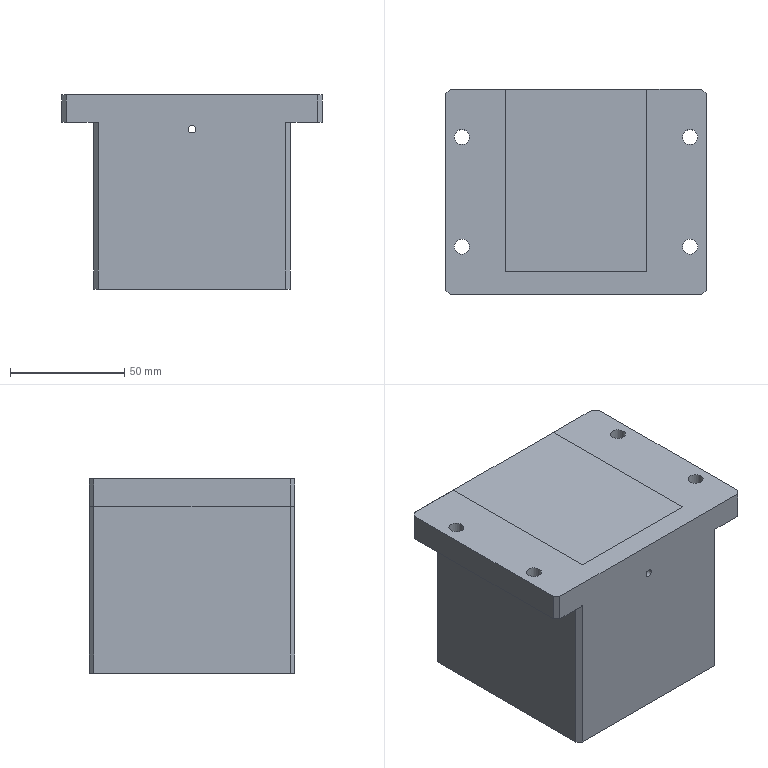Part | 2 solids | 76 faces | box 114 x 90 x 85 mm | volume 955945 mm3 | plane 43 | cylinder 23 | cone 10 | commonest cylinder face diameters 5 x8 6.6 x8 3.3 x2 10 x2 75 x2 55 x1